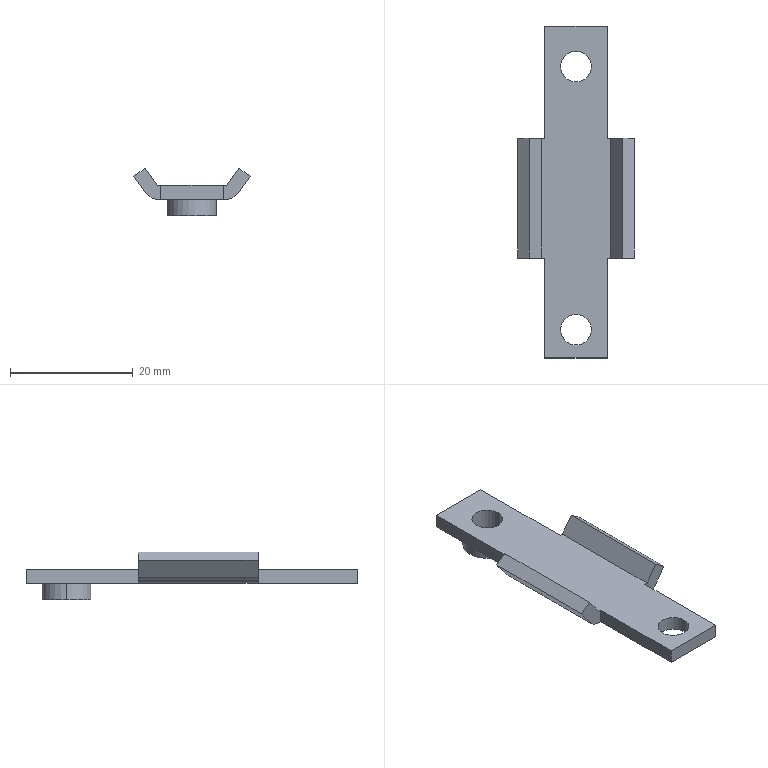Part | STEP file | AC40-04-KSTV-38JNR_AC3009A Spacer Rear Plate(4) | 1 solid | 27 faces | box 18.951 x 54 x 7.773 mm | volume 1709 mm3 | plane 19 | cylinder 8 | commonest cylinder face diameters 5 x4 4.6 x2 8 x2